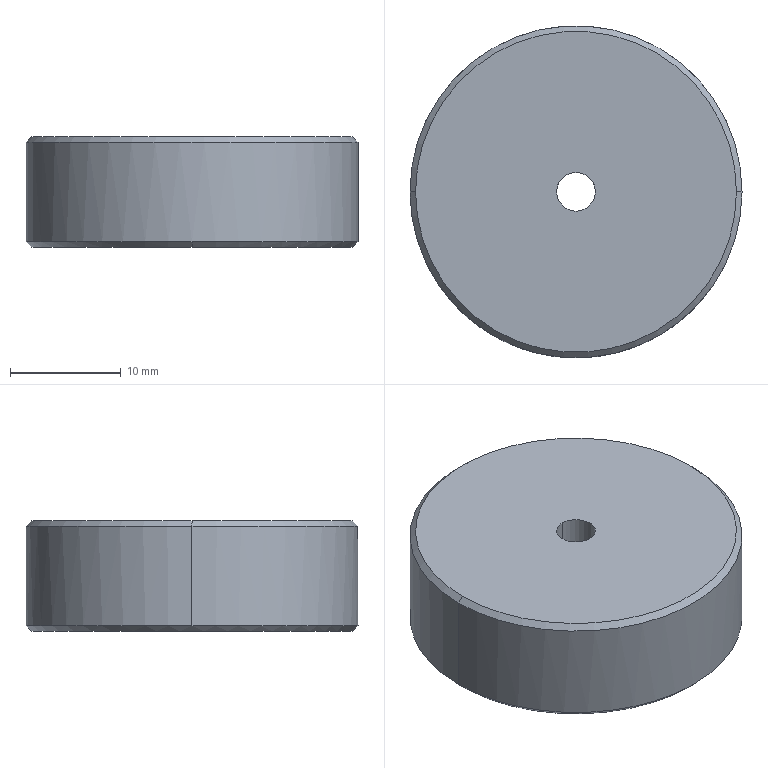Part | STEP file | 04-15 Heat-shrink tube press block | 1 solid | 15 faces | box 30 x 30 x 10 mm | volume 6743 mm3 | cone 6 | cylinder 6 | plane 3 | commonest cylinder face diameters 3.5 x2 8 x2 30 x2
STEP:
#1=CARTESIAN_POINT('',(0.,0.,0.));
#2=DIRECTION('',(0.,0.,1.));
#3=DIRECTION('',(1.,0.,0.));
#4=AXIS2_PLACEMENT_3D('',#1,#2,#3);
#5=CARTESIAN_POINT('',(14.5,0.,0.));
#6=VERTEX_POINT('',#5);
#7=CARTESIAN_POINT('',(-14.5,0.,0.));
#8=VERTEX_POINT('',#7);
#9=CARTESIAN_POINT('',(0.,0.,0.));
#10=DIRECTION('',(0.,0.,1.));
#11=DIRECTION('',(-1.,0.,0.));
#12=AXIS2_PLACEMENT_3D('',#9,#10,#11);
#13=CIRCLE('',#12,14.5);
#14=CARTESIAN_POINT('',(0.,0.,0.));
#15=DIRECTION('',(0.,0.,-1.));
#16=DIRECTION('',(-1.,0.,0.));
#17=AXIS2_PLACEMENT_3D('',#14,#15,#16);
#18=CONICAL_SURFACE('',#17,14.5,0.7854);
#19=CARTESIAN_POINT('',(6.283,0.));
#20=DIRECTION('',(-1.,0.));
#21=VECTOR('',#20,1.);
#22=LINE('',#19,#21);
#23=(GEOMETRIC_REPRESENTATION_CONTEXT(2)PARAMETRIC_REPRESENTATION_CONTEXT()REPRESENTATION_CONTEXT('',''));
#24=DEFINITIONAL_REPRESENTATION('',(#22),#23);
#25=PCURVE('',#18,#24);
#26=CARTESIAN_POINT('',(14.674,-14.674,0.));
#27=DIRECTION('',(0.,0.,-1.));
#28=DIRECTION('',(-1.,0.,0.));
#29=AXIS2_PLACEMENT_3D('',#26,#27,#28);
#30=PLANE('',#29);
#31=CARTESIAN_POINT('',(29.174,14.674));
#32=CARTESIAN_POINT('',(29.174,-10.441));
#33=CARTESIAN_POINT('',(7.424,2.117));
#34=CARTESIAN_POINT('',(-14.326,14.674));
#35=CARTESIAN_POINT('',(7.424,27.231));
#36=CARTESIAN_POINT('',(29.174,39.789));
#37=CARTESIAN_POINT('',(29.174,14.674));
#38=(BOUNDED_CURVE()B_SPLINE_CURVE(2,(#31,#32,#33,#34,#35,#36,#37),.UNSPECIFIED.,.T.,.F.)B_SPLINE_CURVE_WITH_KNOTS((1,2,2,2,2,1),(-2.094,0.,2.094,4.189,6.283,8.378),.UNSPECIFIED.)CURVE()GEOMETRIC_REPRESENTATION_ITEM()RATIONAL_B_SPLINE_CURVE((1.,0.5,1.,0.5,1.,0.5,1.))REPRESENTATION_ITEM(''));
#39=(GEOMETRIC_REPRESENTATION_CONTEXT(2)PARAMETRIC_REPRESENTATION_CONTEXT()REPRESENTATION_CONTEXT('',''));
#40=DEFINITIONAL_REPRESENTATION('',(#38),#39);
#41=PCURVE('',#30,#40);
#42=SURFACE_CURVE('',#13,(#25,#41),.PCURVE_S1.);
#43=EDGE_CURVE('',#6,#8,#42,.T.);
#44=ORIENTED_EDGE('',*,*,#43,.F.);
#45=CARTESIAN_POINT('',(15.,0.,-0.5));
#46=VERTEX_POINT('',#45);
#47=CARTESIAN_POINT('',(14.5,0.,0.));
#48=DIRECTION('',(0.7071,0.,-0.7071));
#49=VECTOR('',#48,1.);
#50=LINE('',#47,#49);
#51=CARTESIAN_POINT('',(3.142,0.));
#52=DIRECTION('',(0.,1.));
#53=VECTOR('',#52,1.);
#54=LINE('',#51,#53);
#55=(GEOMETRIC_REPRESENTATION_CONTEXT(2)PARAMETRIC_REPRESENTATION_CONTEXT()REPRESENTATION_CONTEXT('',''));
#56=DEFINITIONAL_REPRESENTATION('',(#54),#55);
#57=PCURVE('',#18,#56);
#58=CARTESIAN_POINT('',(0.,0.,0.));
#59=DIRECTION('',(0.,0.,-1.));
#60=DIRECTION('',(-1.,0.,0.));
#61=AXIS2_PLACEMENT_3D('',#58,#59,#60);
#62=CONICAL_SURFACE('',#61,14.5,0.7854);
#63=CARTESIAN_POINT('',(3.142,0.));
#64=DIRECTION('',(0.,1.));
#65=VECTOR('',#64,1.);
#66=LINE('',#63,#65);
#67=(GEOMETRIC_REPRESENTATION_CONTEXT(2)PARAMETRIC_REPRESENTATION_CONTEXT()REPRESENTATION_CONTEXT('',''));
#68=DEFINITIONAL_REPRESENTATION('',(#66),#67);
#69=PCURVE('',#62,#68);
#70=SURFACE_CURVE('',#50,(#57,#69),.PCURVE_S1.);
#71=EDGE_CURVE('',#6,#46,#70,.T.);
#72=ORIENTED_EDGE('',*,*,#71,.T.);
#73=CARTESIAN_POINT('',(-15.,0.,-0.5));
#74=VERTEX_POINT('',#73);
#75=CARTESIAN_POINT('',(0.,0.,-0.5));
#76=DIRECTION('',(0.,0.,-1.));
#77=DIRECTION('',(-1.,0.,0.));
#78=AXIS2_PLACEMENT_3D('',#75,#76,#77);
#79=CIRCLE('',#78,15.);
#80=CARTESIAN_POINT('',(0.,0.5));
#81=DIRECTION('',(1.,0.));
#82=VECTOR('',#81,1.);
#83=LINE('',#80,#82);
#84=(GEOMETRIC_REPRESENTATION_CONTEXT(2)PARAMETRIC_REPRESENTATION_CONTEXT()REPRESENTATION_CONTEXT('',''));
#85=DEFINITIONAL_REPRESENTATION('',(#83),#84);
#86=PCURVE('',#18,#85);
#87=CARTESIAN_POINT('',(0.,0.,-9.5));
#88=DIRECTION('',(0.,0.,1.));
#89=DIRECTION('',(1.,0.,0.));
#90=AXIS2_PLACEMENT_3D('',#87,#88,#89);
#91=CYLINDRICAL_SURFACE('',#90,15.);
#92=CARTESIAN_POINT('',(3.142,9.));
#93=DIRECTION('',(-1.,0.));
#94=VECTOR('',#93,1.);
#95=LINE('',#92,#94);
#96=(GEOMETRIC_REPRESENTATION_CONTEXT(2)PARAMETRIC_REPRESENTATION_CONTEXT()REPRESENTATION_CONTEXT('',''));
#97=DEFINITIONAL_REPRESENTATION('',(#95),#96);
#98=PCURVE('',#91,#97);
#99=SURFACE_CURVE('',#79,(#86,#98),.PCURVE_S1.);
#100=EDGE_CURVE('',#74,#46,#99,.T.);
#101=ORIENTED_EDGE('',*,*,#100,.F.);
#102=CARTESIAN_POINT('',(-14.5,0.,0.));
#103=DIRECTION('',(-0.7071,0.,-0.7071));
#104=VECTOR('',#103,1.);
#105=LINE('',#102,#104);
#106=CARTESIAN_POINT('',(0.,0.));
#107=DIRECTION('',(0.,1.));
#108=VECTOR('',#107,1.);
#109=LINE('',#106,#108);
#110=(GEOMETRIC_REPRESENTATION_CONTEXT(2)PARAMETRIC_REPRESENTATION_CONTEXT()REPRESENTATION_CONTEXT('',''));
#111=DEFINITIONAL_REPRESENTATION('',(#109),#110);
#112=PCURVE('',#18,#111);
#113=CARTESIAN_POINT('',(6.283,0.));
#114=DIRECTION('',(0.,1.));
#115=VECTOR('',#114,1.);
#116=LINE('',#113,#115);
#117=(GEOMETRIC_REPRESENTATION_CONTEXT(2)PARAMETRIC_REPRESENTATION_CONTEXT()REPRESENTATION_CONTEXT('',''));
#118=DEFINITIONAL_REPRESENTATION('',(#116),#117);
#119=PCURVE('',#62,#118);
#120=SURFACE_CURVE('',#105,(#112,#119),.PCURVE_S1.);
#121=EDGE_CURVE('',#8,#74,#120,.T.);
#122=ORIENTED_EDGE('',*,*,#121,.F.);
#123=EDGE_LOOP('',(#44,#72,#101,#122));
#124=FACE_BOUND('',#123,.T.);
#125=ADVANCED_FACE('',(#124),#18,.T.);
#126=CARTESIAN_POINT('',(-15.,0.,-9.5));
#127=VERTEX_POINT('',#126);
#128=CARTESIAN_POINT('',(0.,15.,-9.5));
#129=VERTEX_POINT('',#128);
#130=CARTESIAN_POINT('',(0.,0.,-9.5));
#131=DIRECTION('',(0.,0.,-1.));
#132=DIRECTION('',(1.,0.,0.));
#133=AXIS2_PLACEMENT_3D('',#130,#131,#132);
#134=CIRCLE('',#133,15.);
#135=CARTESIAN_POINT('',(6.283,0.));
#136=DIRECTION('',(-1.,0.));
#137=VECTOR('',#136,1.);
#138=LINE('',#135,#137);
#139=(GEOMETRIC_REPRESENTATION_CONTEXT(2)PARAMETRIC_REPRESENTATION_CONTEXT()REPRESENTATION_CONTEXT('',''));
#140=DEFINITIONAL_REPRESENTATION('',(#138),#139);
#141=PCURVE('',#91,#140);
#142=CARTESIAN_POINT('',(0.,0.,-10.));
#143=DIRECTION('',(0.,0.,1.));
#144=DIRECTION('',(0.,-1.,0.));
#145=AXIS2_PLACEMENT_3D('',#142,#143,#144);
#146=CONICAL_SURFACE('',#145,14.5,0.7854);
#147=CARTESIAN_POINT('',(7.854,0.5));
#148=DIRECTION('',(-1.,0.));
#149=VECTOR('',#148,1.);
#150=LINE('',#147,#149);
#151=(GEOMETRIC_REPRESENTATION_CONTEXT(2)PARAMETRIC_REPRESENTATION_CONTEXT()REPRESENTATION_CONTEXT('',''));
#152=DEFINITIONAL_REPRESENTATION('',(#150),#151);
#153=PCURVE('',#146,#152);
#154=SURFACE_CURVE('',#134,(#141,#153),.PCURVE_S1.);
#155=EDGE_CURVE('',#127,#129,#154,.T.);
#156=ORIENTED_EDGE('',*,*,#155,.F.);
#157=CARTESIAN_POINT('',(-15.,0.,-9.5));
#158=DIRECTION('',(0.,0.,1.));
#159=VECTOR('',#158,1.);
#160=LINE('',#157,#159);
#161=CARTESIAN_POINT('',(3.142,0.));
#162=DIRECTION('',(0.,1.));
#163=VECTOR('',#162,1.);
#164=LINE('',#161,#163);
#165=(GEOMETRIC_REPRESENTATION_CONTEXT(2)PARAMETRIC_REPRESENTATION_CONTEXT()REPRESENTATION_CONTEXT('',''));
#166=DEFINITIONAL_REPRESENTATION('',(#164),#165);
#167=PCURVE('',#91,#166);
#168=CARTESIAN_POINT('',(0.,0.,-9.5));
#169=DIRECTION('',(0.,0.,1.));
#170=DIRECTION('',(1.,0.,0.));
#171=AXIS2_PLACEMENT_3D('',#168,#169,#170);
#172=CYLINDRICAL_SURFACE('',#171,15.);
#173=CARTESIAN_POINT('',(3.142,0.));
#174=DIRECTION('',(0.,1.));
#175=VECTOR('',#174,1.);
#176=LINE('',#173,#175);
#177=(GEOMETRIC_REPRESENTATION_CONTEXT(2)PARAMETRIC_REPRESENTATION_CONTEXT()REPRESENTATION_CONTEXT('',''));
#178=DEFINITIONAL_REPRESENTATION('',(#176),#177);
#179=PCURVE('',#172,#178);
#180=SURFACE_CURVE('',#160,(#167,#179),.PCURVE_S1.);
#181=EDGE_CURVE('',#127,#74,#180,.T.);
#182=ORIENTED_EDGE('',*,*,#181,.T.);
#183=ORIENTED_EDGE('',*,*,#100,.T.);
#184=CARTESIAN_POINT('',(15.,0.,-9.5));
#185=VERTEX_POINT('',#184);
#186=CARTESIAN_POINT('',(15.,0.,-9.5));
#187=DIRECTION('',(0.,0.,1.));
#188=VECTOR('',#187,1.);
#189=LINE('',#186,#188);
#190=CARTESIAN_POINT('',(0.,0.));
#191=DIRECTION('',(0.,1.));
#192=VECTOR('',#191,1.);
#193=LINE('',#190,#192);
#194=(GEOMETRIC_REPRESENTATION_CONTEXT(2)PARAMETRIC_REPRESENTATION_CONTEXT()REPRESENTATION_CONTEXT('',''));
#195=DEFINITIONAL_REPRESENTATION('',(#193),#194);
#196=PCURVE('',#91,#195);
#197=CARTESIAN_POINT('',(6.283,0.));
#198=DIRECTION('',(0.,1.));
#199=VECTOR('',#198,1.);
#200=LINE('',#197,#199);
#201=(GEOMETRIC_REPRESENTATION_CONTEXT(2)PARAMETRIC_REPRESENTATION_CONTEXT()REPRESENTATION_CONTEXT('',''));
#202=DEFINITIONAL_REPRESENTATION('',(#200),#201);
#203=PCURVE('',#172,#202);
#204=SURFACE_CURVE('',#189,(#196,#203),.PCURVE_S1.);
#205=EDGE_CURVE('',#185,#46,#204,.T.);
#206=ORIENTED_EDGE('',*,*,#205,.F.);
#207=CARTESIAN_POINT('',(0.,0.,-9.5));
#208=DIRECTION('',(0.,0.,-1.));
#209=DIRECTION('',(1.,0.,0.));
#210=AXIS2_PLACEMENT_3D('',#207,#208,#209);
#211=CIRCLE('',#210,15.);
#212=CARTESIAN_POINT('',(6.283,0.));
#213=DIRECTION('',(-1.,0.));
#214=VECTOR('',#213,1.);
#215=LINE('',#212,#214);
#216=(GEOMETRIC_REPRESENTATION_CONTEXT(2)PARAMETRIC_REPRESENTATION_CONTEXT()REPRESENTATION_CONTEXT('',''));
#217=DEFINITIONAL_REPRESENTATION('',(#215),#216);
#218=PCURVE('',#91,#217);
#219=CARTESIAN_POINT('',(0.,0.,-10.));
#220=DIRECTION('',(0.,0.,1.));
#221=DIRECTION('',(0.,-1.,0.));
#222=AXIS2_PLACEMENT_3D('',#219,#220,#221);
#223=CONICAL_SURFACE('',#222,14.5,0.7854);
#224=CARTESIAN_POINT('',(7.854,0.5));
#225=DIRECTION('',(-1.,0.));
#226=VECTOR('',#225,1.);
#227=LINE('',#224,#226);
#228=(GEOMETRIC_REPRESENTATION_CONTEXT(2)PARAMETRIC_REPRESENTATION_CONTEXT()REPRESENTATION_CONTEXT('',''));
#229=DEFINITIONAL_REPRESENTATION('',(#227),#228);
#230=PCURVE('',#223,#229);
#231=SURFACE_CURVE('',#211,(#218,#230),.PCURVE_S1.);
#232=EDGE_CURVE('',#129,#185,#231,.T.);
#233=ORIENTED_EDGE('',*,*,#232,.F.);
#234=EDGE_LOOP('',(#156,#182,#183,#206,#233));
#235=FACE_BOUND('',#234,.T.);
#236=ADVANCED_FACE('',(#235),#91,.T.);
#237=CARTESIAN_POINT('',(0.,-1.75,-5.));
#238=VERTEX_POINT('',#237);
#239=CARTESIAN_POINT('',(0.,-1.75,0.));
#240=VERTEX_POINT('',#239);
#241=CARTESIAN_POINT('',(0.,-1.75,-5.));
#242=DIRECTION('',(0.,0.,1.));
#243=VECTOR('',#242,1.);
#244=LINE('',#241,#243);
#245=CARTESIAN_POINT('',(0.,0.,-5.));
#246=DIRECTION('',(0.,0.,1.));
#247=DIRECTION('',(0.,-1.,0.));
#248=AXIS2_PLACEMENT_3D('',#245,#246,#247);
#249=CYLINDRICAL_SURFACE('',#248,1.75);
#250=CARTESIAN_POINT('',(6.283,0.));
#251=DIRECTION('',(0.,1.));
#252=VECTOR('',#251,1.);
#253=LINE('',#250,#252);
#254=(GEOMETRIC_REPRESENTATION_CONTEXT(2)PARAMETRIC_REPRESENTATION_CONTEXT()REPRESENTATION_CONTEXT('',''));
#255=DEFINITIONAL_REPRESENTATION('',(#253),#254);
#256=PCURVE('',#249,#255);
#257=CARTESIAN_POINT('',(0.,0.,-5.));
#258=DIRECTION('',(0.,0.,1.));
#259=DIRECTION('',(0.,-1.,0.));
#260=AXIS2_PLACEMENT_3D('',#257,#258,#259);
#261=CYLINDRICAL_SURFACE('',#260,1.75);
#262=CARTESIAN_POINT('',(0.,0.));
#263=DIRECTION('',(0.,1.));
#264=VECTOR('',#263,1.);
#265=LINE('',#262,#264);
#266=(GEOMETRIC_REPRESENTATION_CONTEXT(2)PARAMETRIC_REPRESENTATION_CONTEXT()REPRESENTATION_CONTEXT('',''));
#267=DEFINITIONAL_REPRESENTATION('',(#265),#266);
#268=PCURVE('',#261,#267);
#269=SURFACE_CURVE('',#244,(#256,#268),.PCURVE_S1.);
#270=EDGE_CURVE('',#238,#240,#269,.T.);
#271=ORIENTED_EDGE('',*,*,#270,.T.);
#272=CARTESIAN_POINT('',(0.,1.75,0.));
#273=VERTEX_POINT('',#272);
#274=CARTESIAN_POINT('',(0.,0.,0.));
#275=DIRECTION('',(0.,0.,1.));
#276=DIRECTION('',(0.,-1.,0.));
#277=AXIS2_PLACEMENT_3D('',#274,#275,#276);
#278=CIRCLE('',#277,1.75);
#279=CARTESIAN_POINT('',(0.,5.));
#280=DIRECTION('',(1.,0.));
#281=VECTOR('',#280,1.);
#282=LINE('',#279,#281);
#283=(GEOMETRIC_REPRESENTATION_CONTEXT(2)PARAMETRIC_REPRESENTATION_CONTEXT()REPRESENTATION_CONTEXT('',''));
#284=DEFINITIONAL_REPRESENTATION('',(#282),#283);
#285=PCURVE('',#249,#284);
#286=CARTESIAN_POINT('',(14.674,12.924));
#287=CARTESIAN_POINT('',(11.643,12.924));
#288=CARTESIAN_POINT('',(13.158,15.549));
#289=CARTESIAN_POINT('',(14.674,18.174));
#290=CARTESIAN_POINT('',(16.19,15.549));
#291=CARTESIAN_POINT('',(17.705,12.924));
#292=CARTESIAN_POINT('',(14.674,12.924));
#293=(BOUNDED_CURVE()B_SPLINE_CURVE(2,(#286,#287,#288,#289,#290,#291,#292),.UNSPECIFIED.,.T.,.F.)B_SPLINE_CURVE_WITH_KNOTS((1,2,2,2,2,1),(-2.094,0.,2.094,4.189,6.283,8.378),.UNSPECIFIED.)CURVE()GEOMETRIC_REPRESENTATION_ITEM()RATIONAL_B_SPLINE_CURVE((1.,0.5,1.,0.5,1.,0.5,1.))REPRESENTATION_ITEM(''));
#294=(GEOMETRIC_REPRESENTATION_CONTEXT(2)PARAMETRIC_REPRESENTATION_CONTEXT()REPRESENTATION_CONTEXT('',''));
#295=DEFINITIONAL_REPRESENTATION('',(#293),#294);
#296=PCURVE('',#30,#295);
#297=SURFACE_CURVE('',#278,(#285,#296),.PCURVE_S1.);
#298=EDGE_CURVE('',#273,#240,#297,.T.);
#299=ORIENTED_EDGE('',*,*,#298,.F.);
#300=CARTESIAN_POINT('',(0.,1.75,-5.));
#301=VERTEX_POINT('',#300);
#302=CARTESIAN_POINT('',(0.,1.75,-5.));
#303=DIRECTION('',(0.,0.,1.));
#304=VECTOR('',#303,1.);
#305=LINE('',#302,#304);
#306=CARTESIAN_POINT('',(3.142,0.));
#307=DIRECTION('',(0.,1.));
#308=VECTOR('',#307,1.);
#309=LINE('',#306,#308);
#310=(GEOMETRIC_REPRESENTATION_CONTEXT(2)PARAMETRIC_REPRESENTATION_CONTEXT()REPRESENTATION_CONTEXT('',''));
#311=DEFINITIONAL_REPRESENTATION('',(#309),#310);
#312=PCURVE('',#249,#311);
#313=CARTESIAN_POINT('',(3.142,0.));
#314=DIRECTION('',(0.,1.));
#315=VECTOR('',#314,1.);
#316=LINE('',#313,#315);
#317=(GEOMETRIC_REPRESENTATION_CONTEXT(2)PARAMETRIC_REPRESENTATION_CONTEXT()REPRESENTATION_CONTEXT('',''));
#318=DEFINITIONAL_REPRESENTATION('',(#316),#317);
#319=PCURVE('',#261,#318);
#320=SURFACE_CURVE('',#305,(#312,#319),.PCURVE_S1.);
#321=EDGE_CURVE('',#301,#273,#320,.T.);
#322=ORIENTED_EDGE('',*,*,#321,.F.);
#323=CARTESIAN_POINT('',(0.,0.,-5.));
#324=DIRECTION('',(0.,0.,-1.));
#325=DIRECTION('',(0.,-1.,0.));
#326=AXIS2_PLACEMENT_3D('',#323,#324,#325);
#327=CIRCLE('',#326,1.75);
#328=CARTESIAN_POINT('',(6.283,0.));
#329=DIRECTION('',(-1.,0.));
#330=VECTOR('',#329,1.);
#331=LINE('',#328,#330);
#332=(GEOMETRIC_REPRESENTATION_CONTEXT(2)PARAMETRIC_REPRESENTATION_CONTEXT()REPRESENTATION_CONTEXT('',''));
#333=DEFINITIONAL_REPRESENTATION('',(#331),#332);
#334=PCURVE('',#249,#333);
#335=CARTESIAN_POINT('',(-4.048,-4.048,-5.));
#336=DIRECTION('',(0.,0.,1.));
#337=DIRECTION('',(1.,0.,0.));
#338=AXIS2_PLACEMENT_3D('',#335,#336,#337);
#339=PLANE('',#338);
#340=CARTESIAN_POINT('',(4.048,2.298));
#341=CARTESIAN_POINT('',(1.017,2.298));
#342=CARTESIAN_POINT('',(2.532,4.923));
#343=CARTESIAN_POINT('',(4.048,7.548));
#344=CARTESIAN_POINT('',(5.564,4.923));
#345=CARTESIAN_POINT('',(7.079,2.298));
#346=CARTESIAN_POINT('',(4.048,2.298));
#347=(BOUNDED_CURVE()B_SPLINE_CURVE(2,(#340,#341,#342,#343,#344,#345,#346),.UNSPECIFIED.,.T.,.F.)B_SPLINE_CURVE_WITH_KNOTS((1,2,2,2,2,1),(-2.094,0.,2.094,4.189,6.283,8.378),.UNSPECIFIED.)CURVE()GEOMETRIC_REPRESENTATION_ITEM()RATIONAL_B_SPLINE_CURVE((1.,0.5,1.,0.5,1.,0.5,1.))REPRESENTATION_ITEM(''));
#348=(GEOMETRIC_REPRESENTATION_CONTEXT(2)PARAMETRIC_REPRESENTATION_CONTEXT()REPRESENTATION_CONTEXT('',''));
#349=DEFINITIONAL_REPRESENTATION('',(#347),#348);
#350=PCURVE('',#339,#349);
#351=SURFACE_CURVE('',#327,(#334,#350),.PCURVE_S1.);
#352=EDGE_CURVE('',#238,#301,#351,.T.);
#353=ORIENTED_EDGE('',*,*,#352,.F.);
#354=EDGE_LOOP('',(#271,#299,#322,#353));
#355=FACE_BOUND('',#354,.F.);
#356=ADVANCED_FACE('',(#355),#249,.F.);
#357=CARTESIAN_POINT('',(0.,14.5,-10.));
#358=VERTEX_POINT('',#357);
#359=CARTESIAN_POINT('',(0.,-14.5,-10.));
#360=VERTEX_POINT('',#359);
#361=CARTESIAN_POINT('',(0.,0.,-10.));
#362=DIRECTION('',(0.,0.,-1.));
#363=DIRECTION('',(0.,-1.,0.));
#364=AXIS2_PLACEMENT_3D('',#361,#362,#363);
#365=CIRCLE('',#364,14.5);
#366=CARTESIAN_POINT('',(6.283,0.));
#367=DIRECTION('',(-1.,0.));
#368=VECTOR('',#367,1.);
#369=LINE('',#366,#368);
#370=(GEOMETRIC_REPRESENTATION_CONTEXT(2)PARAMETRIC_REPRESENTATION_CONTEXT()REPRESENTATION_CONTEXT('',''));
#371=DEFINITIONAL_REPRESENTATION('',(#369),#370);
#372=PCURVE('',#223,#371);
#373=CARTESIAN_POINT('',(-14.674,-14.674,-10.));
#374=DIRECTION('',(0.,0.,1.));
#375=DIRECTION('',(1.,0.,0.));
#376=AXIS2_PLACEMENT_3D('',#373,#374,#375);
#377=PLANE('',#376);
#378=CARTESIAN_POINT('',(14.674,0.174));
#379=CARTESIAN_POINT('',(-10.441,0.174));
#380=CARTESIAN_POINT('',(2.117,21.924));
#381=CARTESIAN_POINT('',(14.674,43.674));
#382=CARTESIAN_POINT('',(27.231,21.924));
#383=CARTESIAN_POINT('',(39.789,0.174));
#384=CARTESIAN_POINT('',(14.674,0.174));
#385=(BOUNDED_CURVE()B_SPLINE_CURVE(2,(#378,#379,#380,#381,#382,#383,#384),.UNSPECIFIED.,.T.,.F.)B_SPLINE_CURVE_WITH_KNOTS((1,2,2,2,2,1),(-2.094,0.,2.094,4.189,6.283,8.378),.UNSPECIFIED.)CURVE()GEOMETRIC_REPRESENTATION_ITEM()RATIONAL_B_SPLINE_CURVE((1.,0.5,1.,0.5,1.,0.5,1.))REPRESENTATION_ITEM(''));
#386=(GEOMETRIC_REPRESENTATION_CONTEXT(2)PARAMETRIC_REPRESENTATION_CONTEXT()REPRESENTATION_CONTEXT('',''));
#387=DEFINITIONAL_REPRESENTATION('',(#385),#386);
#388=PCURVE('',#377,#387);
#389=SURFACE_CURVE('',#365,(#372,#388),.PCURVE_S1.);
#390=EDGE_CURVE('',#358,#360,#389,.T.);
#391=ORIENTED_EDGE('',*,*,#390,.F.);
#392=CARTESIAN_POINT('',(0.,14.5,-10.));
#393=DIRECTION('',(0.,0.7071,0.7071));
#394=VECTOR('',#393,1.);
#395=LINE('',#392,#394);
#396=CARTESIAN_POINT('',(3.142,0.));
#397=DIRECTION('',(0.,1.));
#398=VECTOR('',#397,1.);
#399=LINE('',#396,#398);
#400=(GEOMETRIC_REPRESENTATION_CONTEXT(2)PARAMETRIC_REPRESENTATION_CONTEXT()REPRESENTATION_CONTEXT('',''));
#401=DEFINITIONAL_REPRESENTATION('',(#399),#400);
#402=PCURVE('',#223,#401);
#403=CARTESIAN_POINT('',(3.142,0.));
#404=DIRECTION('',(0.,1.));
#405=VECTOR('',#404,1.);
#406=LINE('',#403,#405);
#407=(GEOMETRIC_REPRESENTATION_CONTEXT(2)PARAMETRIC_REPRESENTATION_CONTEXT()REPRESENTATION_CONTEXT('',''));
#408=DEFINITIONAL_REPRESENTATION('',(#406),#407);
#409=PCURVE('',#146,#408);
#410=SURFACE_CURVE('',#395,(#402,#409),.PCURVE_S1.);
#411=EDGE_CURVE('',#358,#129,#410,.T.);
#412=ORIENTED_EDGE('',*,*,#411,.T.);
#413=ORIENTED_EDGE('',*,*,#232,.T.);
#414=CARTESIAN_POINT('',(0.,-15.,-9.5));
#415=VERTEX_POINT('',#414);
#416=CARTESIAN_POINT('',(0.,0.,-9.5));
#417=DIRECTION('',(0.,0.,-1.));
#418=DIRECTION('',(1.,0.,0.));
#419=AXIS2_PLACEMENT_3D('',#416,#417,#418);
#420=CIRCLE('',#419,15.);
#421=CARTESIAN_POINT('',(1.571,0.5));
#422=DIRECTION('',(-1.,0.));
#423=VECTOR('',#422,1.);
#424=LINE('',#421,#423);
#425=(GEOMETRIC_REPRESENTATION_CONTEXT(2)PARAMETRIC_REPRESENTATION_CONTEXT()REPRESENTATION_CONTEXT('',''));
#426=DEFINITIONAL_REPRESENTATION('',(#424),#425);
#427=PCURVE('',#223,#426);
#428=CARTESIAN_POINT('',(6.283,0.));
#429=DIRECTION('',(-1.,0.));
#430=VECTOR('',#429,1.);
#431=LINE('',#428,#430);
#432=(GEOMETRIC_REPRESENTATION_CONTEXT(2)PARAMETRIC_REPRESENTATION_CONTEXT()REPRESENTATION_CONTEXT('',''));
#433=DEFINITIONAL_REPRESENTATION('',(#431),#432);
#434=PCURVE('',#172,#433);
#435=SURFACE_CURVE('',#420,(#427,#434),.PCURVE_S1.);
#436=EDGE_CURVE('',#185,#415,#435,.T.);
#437=ORIENTED_EDGE('',*,*,#436,.T.);
#438=CARTESIAN_POINT('',(0.,-14.5,-10.));
#439=DIRECTION('',(0.,-0.7071,0.7071));
#440=VECTOR('',#439,1.);
#441=LINE('',#438,#440);
#442=CARTESIAN_POINT('',(0.,0.));
#443=DIRECTION('',(0.,1.));
#444=VECTOR('',#443,1.);
#445=LINE('',#442,#444);
#446=(GEOMETRIC_REPRESENTATION_CONTEXT(2)PARAMETRIC_REPRESENTATION_CONTEXT()REPRESENTATION_CONTEXT('',''));
#447=DEFINITIONAL_REPRESENTATION('',(#445),#446);
#448=PCURVE('',#223,#447);
#449=CARTESIAN_POINT('',(6.283,0.));
#450=DIRECTION('',(0.,1.));
#451=VECTOR('',#450,1.);
#452=LINE('',#449,#451);
#453=(GEOMETRIC_REPRESENTATION_CONTEXT(2)PARAMETRIC_REPRESENTATION_CONTEXT()REPRESENTATION_CONTEXT('',''));
#454=DEFINITIONAL_REPRESENTATION('',(#452),#453);
#455=PCURVE('',#146,#454);
#456=SURFACE_CURVE('',#441,(#448,#455),.PCURVE_S1.);
#457=EDGE_CURVE('',#360,#415,#456,.T.);
#458=ORIENTED_EDGE('',*,*,#457,.F.);
#459=EDGE_LOOP('',(#391,#412,#413,#437,#458));
#460=FACE_BOUND('',#459,.T.);
#461=ADVANCED_FACE('',(#460),#223,.T.);
#462=CARTESIAN_POINT('',(4.,0.,-9.5));
#463=VERTEX_POINT('',#462);
#464=CARTESIAN_POINT('',(4.,0.,-5.));
#465=VERTEX_POINT('',#464);
#466=CARTESIAN_POINT('',(4.,0.,-9.5));
#467=DIRECTION('',(0.,0.,1.));
#468=VECTOR('',#467,1.);
#469=LINE('',#466,#468);
#470=CARTESIAN_POINT('',(0.,0.,-9.5));
#471=DIRECTION('',(0.,0.,1.));
#472=DIRECTION('',(1.,0.,0.));
#473=AXIS2_PLACEMENT_3D('',#470,#471,#472);
#474=CYLINDRICAL_SURFACE('',#473,4.);
#475=CARTESIAN_POINT('',(6.283,0.));
#476=DIRECTION('',(0.,1.));
#477=VECTOR('',#476,1.);
#478=LINE('',#475,#477);
#479=(GEOMETRIC_REPRESENTATION_CONTEXT(2)PARAMETRIC_REPRESENTATION_CONTEXT()REPRESENTATION_CONTEXT('',''));
#480=DEFINITIONAL_REPRESENTATION('',(#478),#479);
#481=PCURVE('',#474,#480);
#482=CARTESIAN_POINT('',(0.,0.,-9.5));
#483=DIRECTION('',(0.,0.,1.));
#484=DIRECTION('',(1.,0.,0.));
#485=AXIS2_PLACEMENT_3D('',#482,#483,#484);
#486=CYLINDRICAL_SURFACE('',#485,4.);
#487=CARTESIAN_POINT('',(0.,0.));
#488=DIRECTION('',(0.,1.));
#489=VECTOR('',#488,1.);
#490=LINE('',#487,#489);
#491=(GEOMETRIC_REPRESENTATION_CONTEXT(2)PARAMETRIC_REPRESENTATION_CONTEXT()REPRESENTATION_CONTEXT('',''));
#492=DEFINITIONAL_REPRESENTATION('',(#490),#491);
#493=PCURVE('',#486,#492);
#494=SURFACE_CURVE('',#469,(#481,#493),.PCURVE_S1.);
#495=EDGE_CURVE('',#463,#465,#494,.T.);
#496=ORIENTED_EDGE('',*,*,#495,.T.);
#497=CARTESIAN_POINT('',(-4.,0.,-5.));
#498=VERTEX_POINT('',#497);
#499=CARTESIAN_POINT('',(0.,0.,-5.));
#500=DIRECTION('',(0.,0.,1.));
#501=DIRECTION('',(1.,0.,0.));
#502=AXIS2_PLACEMENT_3D('',#499,#500,#501);
#503=CIRCLE('',#502,4.);
#504=CARTESIAN_POINT('',(0.,4.5));
#505=DIRECTION('',(1.,0.));
#506=VECTOR('',#505,1.);
#507=LINE('',#504,#506);
#508=(GEOMETRIC_REPRESENTATION_CONTEXT(2)PARAMETRIC_REPRESENTATION_CONTEXT()REPRESENTATION_CONTEXT('',''));
#509=DEFINITIONAL_REPRESENTATION('',(#507),#508);
#510=PCURVE('',#474,#509);
#511=CARTESIAN_POINT('',(4.048,4.048));
#512=DIRECTION('',(1.,0.));
#513=AXIS2_PLACEMENT_2D('',#511,#512);
#514=CIRCLE('',#513,4.);
#515=(GEOMETRIC_REPRESENTATION_CONTEXT(2)PARAMETRIC_REPRESENTATION_CONTEXT()REPRESENTATION_CONTEXT('',''));
#516=DEFINITIONAL_REPRESENTATION('',(#514),#515);
#517=PCURVE('',#339,#516);
#518=SURFACE_CURVE('',#503,(#510,#517),.PCURVE_S1.);
#519=EDGE_CURVE('',#498,#465,#518,.T.);
#520=ORIENTED_EDGE('',*,*,#519,.F.);
#521=CARTESIAN_POINT('',(-4.,0.,-9.5));
#522=VERTEX_POINT('',#521);
#523=CARTESIAN_POINT('',(-4.,0.,-9.5));
#524=DIRECTION('',(0.,0.,1.));
#525=VECTOR('',#524,1.);
#526=LINE('',#523,#525);
#527=CARTESIAN_POINT('',(3.142,0.));
#528=DIRECTION('',(0.,1.));
#529=VECTOR('',#528,1.);
#530=LINE('',#527,#529);
#531=(GEOMETRIC_REPRESENTATION_CONTEXT(2)PARAMETRIC_REPRESENTATION_CONTEXT()REPRESENTATION_CONTEXT('',''));
#532=DEFINITIONAL_REPRESENTATION('',(#530),#531);
#533=PCURVE('',#474,#532);
#534=CARTESIAN_POINT('',(3.142,0.));
#535=DIRECTION('',(0.,1.));
#536=VECTOR('',#535,1.);
#537=LINE('',#534,#536);
#538=(GEOMETRIC_REPRESENTATION_CONTEXT(2)PARAMETRIC_REPRESENTATION_CONTEXT()REPRESENTATION_CONTEXT('',''));
#539=DEFINITIONAL_REPRESENTATION('',(#537),#538);
#540=PCURVE('',#486,#539);
#541=SURFACE_CURVE('',#526,(#533,#540),.PCURVE_S1.);
#542=EDGE_CURVE('',#522,#498,#541,.T.);
#543=ORIENTED_EDGE('',*,*,#542,.F.);
#544=CARTESIAN_POINT('',(0.,0.,-9.5));
#545=DIRECTION('',(0.,0.,-1.));
#546=DIRECTION('',(1.,0.,0.));
#547=AXIS2_PLACEMENT_3D('',#544,#545,#546);
#548=CIRCLE('',#547,4.);
#549=CARTESIAN_POINT('',(6.283,0.));
#550=DIRECTION('',(-1.,0.));
#551=VECTOR('',#550,1.);
#552=LINE('',#549,#551);
#553=(GEOMETRIC_REPRESENTATION_CONTEXT(2)PARAMETRIC_REPRESENTATION_CONTEXT()REPRESENTATION_CONTEXT('',''));
#554=DEFINITIONAL_REPRESENTATION('',(#552),#553);
#555=PCURVE('',#474,#554);
#556=CARTESIAN_POINT('',(0.,0.,-9.5));
#557=DIRECTION('',(0.,0.,-1.));
#558=DIRECTION('',(-1.,0.,0.));
#559=AXIS2_PLACEMENT_3D('',#556,#557,#558);
#560=CONICAL_SURFACE('',#559,4.,0.7854);
#561=CARTESIAN_POINT('',(3.142,0.));
#562=DIRECTION('',(1.,0.));
#563=VECTOR('',#562,1.);
#564=LINE('',#561,#563);
#565=(GEOMETRIC_REPRESENTATION_CONTEXT(2)PARAMETRIC_REPRESENTATION_CONTEXT()REPRESENTATION_CONTEXT('',''));
#566=DEFINITIONAL_REPRESENTATION('',(#564),#565);
#567=PCURVE('',#560,#566);
#568=SURFACE_CURVE('',#548,(#555,#567),.PCURVE_S1.);
#569=EDGE_CURVE('',#463,#522,#568,.T.);
#570=ORIENTED_EDGE('',*,*,#569,.F.);
#571=EDGE_LOOP('',(#496,#520,#543,#570));
#572=FACE_BOUND('',#571,.F.);
#573=ADVANCED_FACE('',(#572),#474,.F.);
#574=CARTESIAN_POINT('',(-4.5,0.,-10.));
#575=VERTEX_POINT('',#574);
#576=CARTESIAN_POINT('',(-4.,0.,-9.5));
#577=DIRECTION('',(-0.7071,0.,-0.7071));
#578=VECTOR('',#577,1.);
#579=LINE('',#576,#578);
#580=CARTESIAN_POINT('',(6.283,0.));
#581=DIRECTION('',(0.,1.));
#582=VECTOR('',#581,1.);
#583=LINE('',#580,#582);
#584=(GEOMETRIC_REPRESENTATION_CONTEXT(2)PARAMETRIC_REPRESENTATION_CONTEXT()REPRESENTATION_CONTEXT('',''));
#585=DEFINITIONAL_REPRESENTATION('',(#583),#584);
#586=PCURVE('',#560,#585);
#587=CARTESIAN_POINT('',(0.,0.,-9.5));
#588=DIRECTION('',(0.,0.,-1.));
#589=DIRECTION('',(-1.,0.,0.));
#590=AXIS2_PLACEMENT_3D('',#587,#588,#589);
#591=CONICAL_SURFACE('',#590,4.,0.7854);
#592=CARTESIAN_POINT('',(0.,0.));
#593=DIRECTION('',(0.,1.));
#594=VECTOR('',#593,1.);
#595=LINE('',#592,#594);
#596=(GEOMETRIC_REPRESENTATION_CONTEXT(2)PARAMETRIC_REPRESENTATION_CONTEXT()REPRESENTATION_CONTEXT('',''));
#597=DEFINITIONAL_REPRESENTATION('',(#595),#596);
#598=PCURVE('',#591,#597);
#599=SURFACE_CURVE('',#579,(#586,#598),.PCURVE_S1.);
#600=EDGE_CURVE('',#522,#575,#599,.T.);
#601=ORIENTED_EDGE('',*,*,#600,.T.);
#602=CARTESIAN_POINT('',(4.5,0.,-10.));
#603=VERTEX_POINT('',#602);
#604=CARTESIAN_POINT('',(0.,0.,-10.));
#605=DIRECTION('',(0.,0.,-1.));
#606=DIRECTION('',(-1.,0.,0.));
#607=AXIS2_PLACEMENT_3D('',#604,#605,#606);
#608=CIRCLE('',#607,4.5);
#609=CARTESIAN_POINT('',(0.,0.5));
#610=DIRECTION('',(1.,0.));
#611=VECTOR('',#610,1.);
#612=LINE('',#609,#611);
#613=(GEOMETRIC_REPRESENTATION_CONTEXT(2)PARAMETRIC_REPRESENTATION_CONTEXT()REPRESENTATION_CONTEXT('',''));
#614=DEFINITIONAL_REPRESENTATION('',(#612),#613);
#615=PCURVE('',#560,#614);
#616=CARTESIAN_POINT('',(10.174,14.674));
#617=CARTESIAN_POINT('',(10.174,22.468));
#618=CARTESIAN_POINT('',(16.924,18.571));
#619=CARTESIAN_POINT('',(23.674,14.674));
#620=CARTESIAN_POINT('',(16.924,10.777));
#621=CARTESIAN_POINT('',(10.174,6.88));
#622=CARTESIAN_POINT('',(10.174,14.674));
#623=(BOUNDED_CURVE()B_SPLINE_CURVE(2,(#616,#617,#618,#619,#620,#621,#622),.UNSPECIFIED.,.T.,.F.)B_SPLINE_CURVE_WITH_KNOTS((1,2,2,2,2,1),(-2.094,0.,2.094,4.189,6.283,8.378),.UNSPECIFIED.)CURVE()GEOMETRIC_REPRESENTATION_ITEM()RATIONAL_B_SPLINE_CURVE((1.,0.5,1.,0.5,1.,0.5,1.))REPRESENTATION_ITEM(''));
#624=(GEOMETRIC_REPRESENTATION_CONTEXT(2)PARAMETRIC_REPRESENTATION_CONTEXT()REPRESENTATION_CONTEXT('',''));
#625=DEFINITIONAL_REPRESENTATION('',(#623),#624);
#626=PCURVE('',#377,#625);
#627=SURFACE_CURVE('',#608,(#615,#626),.PCURVE_S1.);
#628=EDGE_CURVE('',#603,#575,#627,.T.);
#629=ORIENTED_EDGE('',*,*,#628,.F.);
#630=CARTESIAN_POINT('',(4.,0.,-9.5));
#631=DIRECTION('',(0.7071,0.,-0.7071));
#632=VECTOR('',#631,1.);
#633=LINE('',#630,#632);
#634=CARTESIAN_POINT('',(3.142,0.));
#635=DIRECTION('',(0.,1.));
#636=VECTOR('',#635,1.);
#637=LINE('',#634,#636);
#638=(GEOMETRIC_REPRESENTATION_CONTEXT(2)PARAMETRIC_REPRESENTATION_CONTEXT()REPRESENTATION_CONTEXT('',''));
#639=DEFINITIONAL_REPRESENTATION('',(#637),#638);
#640=PCURVE('',#560,#639);
#641=CARTESIAN_POINT('',(3.142,0.));
#642=DIRECTION('',(0.,1.));
#643=VECTOR('',#642,1.);
#644=LINE('',#641,#643);
#645=(GEOMETRIC_REPRESENTATION_CONTEXT(2)PARAMETRIC_REPRESENTATION_CONTEXT()REPRESENTATION_CONTEXT('',''));
#646=DEFINITIONAL_REPRESENTATION('',(#644),#645);
#647=PCURVE('',#591,#646);
#648=SURFACE_CURVE('',#633,(#640,#647),.PCURVE_S1.);
#649=EDGE_CURVE('',#463,#603,#648,.T.);
#650=ORIENTED_EDGE('',*,*,#649,.F.);
#651=ORIENTED_EDGE('',*,*,#569,.T.);
#652=EDGE_LOOP('',(#601,#629,#650,#651));
#653=FACE_BOUND('',#652,.F.);
#654=ADVANCED_FACE('',(#653),#560,.F.);
#655=ORIENTED_EDGE('',*,*,#71,.F.);
#656=CARTESIAN_POINT('',(0.,0.,0.));
#657=DIRECTION('',(0.,0.,1.));
#658=DIRECTION('',(-1.,0.,0.));
#659=AXIS2_PLACEMENT_3D('',#656,#657,#658);
#660=CIRCLE('',#659,14.5);
#661=CARTESIAN_POINT('',(6.283,0.));
#662=DIRECTION('',(-1.,0.));
#663=VECTOR('',#662,1.);
#664=LINE('',#661,#663);
#665=(GEOMETRIC_REPRESENTATION_CONTEXT(2)PARAMETRIC_REPRESENTATION_CONTEXT()REPRESENTATION_CONTEXT('',''));
#666=DEFINITIONAL_REPRESENTATION('',(#664),#665);
#667=PCURVE('',#62,#666);
#668=CARTESIAN_POINT('',(29.174,14.674));
#669=CARTESIAN_POINT('',(29.174,-10.441));
#670=CARTESIAN_POINT('',(7.424,2.117));
#671=CARTESIAN_POINT('',(-14.326,14.674));
#672=CARTESIAN_POINT('',(7.424,27.231));
#673=CARTESIAN_POINT('',(29.174,39.789));
#674=CARTESIAN_POINT('',(29.174,14.674));
#675=(BOUNDED_CURVE()B_SPLINE_CURVE(2,(#668,#669,#670,#671,#672,#673,#674),.UNSPECIFIED.,.T.,.F.)B_SPLINE_CURVE_WITH_KNOTS((1,2,2,2,2,1),(-2.094,0.,2.094,4.189,6.283,8.378),.UNSPECIFIED.)CURVE()GEOMETRIC_REPRESENTATION_ITEM()RATIONAL_B_SPLINE_CURVE((1.,0.5,1.,0.5,1.,0.5,1.))REPRESENTATION_ITEM(''));
#676=(GEOMETRIC_REPRESENTATION_CONTEXT(2)PARAMETRIC_REPRESENTATION_CONTEXT()REPRESENTATION_CONTEXT('',''));
#677=DEFINITIONAL_REPRESENTATION('',(#675),#676);
#678=PCURVE('',#30,#677);
#679=SURFACE_CURVE('',#660,(#667,#678),.PCURVE_S1.);
#680=EDGE_CURVE('',#8,#6,#679,.T.);
#681=ORIENTED_EDGE('',*,*,#680,.F.);
#682=ORIENTED_EDGE('',*,*,#121,.T.);
#683=CARTESIAN_POINT('',(0.,0.,-0.5));
#684=DIRECTION('',(0.,0.,-1.));
#685=DIRECTION('',(-1.,0.,0.));
#686=AXIS2_PLACEMENT_3D('',#683,#684,#685);
#687=CIRCLE('',#686,15.);
#688=CARTESIAN_POINT('',(0.,0.5));
#689=DIRECTION('',(1.,0.));
#690=VECTOR('',#689,1.);
#691=LINE('',#688,#690);
#692=(GEOMETRIC_REPRESENTATION_CONTEXT(2)PARAMETRIC_REPRESENTATION_CONTEXT()REPRESENTATION_CONTEXT('',''));
#693=DEFINITIONAL_REPRESENTATION('',(#691),#692);
#694=PCURVE('',#62,#693);
#695=CARTESIAN_POINT('',(9.425,9.));
#696=DIRECTION('',(-1.,0.));
#697=VECTOR('',#696,1.);
#698=LINE('',#695,#697);
#699=(GEOMETRIC_REPRESENTATION_CONTEXT(2)PARAMETRIC_REPRESENTATION_CONTEXT()REPRESENTATION_CONTEXT('',''));
#700=DEFINITIONAL_REPRESENTATION('',(#698),#699);
#701=PCURVE('',#172,#700);
#702=SURFACE_CURVE('',#687,(#694,#701),.PCURVE_S1.);
#703=EDGE_CURVE('',#46,#74,#702,.T.);
#704=ORIENTED_EDGE('',*,*,#703,.F.);
#705=EDGE_LOOP('',(#655,#681,#682,#704));
#706=FACE_BOUND('',#705,.T.);
#707=ADVANCED_FACE('',(#706),#62,.T.);
#708=CARTESIAN_POINT('',(0.,0.,0.));
#709=DIRECTION('',(0.,0.,1.));
#710=DIRECTION('',(0.,-1.,0.));
#711=AXIS2_PLACEMENT_3D('',#708,#709,#710);
#712=CIRCLE('',#711,1.75);
#713=CARTESIAN_POINT('',(14.674,12.924));
#714=CARTESIAN_POINT('',(11.643,12.924));
#715=CARTESIAN_POINT('',(13.158,15.549));
#716=CARTESIAN_POINT('',(14.674,18.174));
#717=CARTESIAN_POINT('',(16.19,15.549));
#718=CARTESIAN_POINT('',(17.705,12.924));
#719=CARTESIAN_POINT('',(14.674,12.924));
#720=(BOUNDED_CURVE()B_SPLINE_CURVE(2,(#713,#714,#715,#716,#717,#718,#719),.UNSPECIFIED.,.T.,.F.)B_SPLINE_CURVE_WITH_KNOTS((1,2,2,2,2,1),(-2.094,0.,2.094,4.189,6.283,8.378),.UNSPECIFIED.)CURVE()GEOMETRIC_REPRESENTATION_ITEM()RATIONAL_B_SPLINE_CURVE((1.,0.5,1.,0.5,1.,0.5,1.))REPRESENTATION_ITEM(''));
#721=(GEOMETRIC_REPRESENTATION_CONTEXT(2)PARAMETRIC_REPRESENTATION_CONTEXT()REPRESENTATION_CONTEXT('',''));
#722=DEFINITIONAL_REPRESENTATION('',(#720),#721);
#723=PCURVE('',#30,#722);
#724=CARTESIAN_POINT('',(0.,5.));
#725=DIRECTION('',(1.,0.));
#726=VECTOR('',#725,1.);
#727=LINE('',#724,#726);
#728=(GEOMETRIC_REPRESENTATION_CONTEXT(2)PARAMETRIC_REPRESENTATION_CONTEXT()REPRESENTATION_CONTEXT('',''));
#729=DEFINITIONAL_REPRESENTATION('',(#727),#728);
#730=PCURVE('',#261,#729);
#731=SURFACE_CURVE('',#712,(#723,#730),.PCURVE_S1.);
#732=EDGE_CURVE('',#240,#273,#731,.T.);
#733=ORIENTED_EDGE('',*,*,#732,.F.);
#734=ORIENTED_EDGE('',*,*,#298,.F.);
#735=EDGE_LOOP('',(#733,#734));
#736=FACE_BOUND('',#735,.T.);
#737=ORIENTED_EDGE('',*,*,#680,.T.);
#738=ORIENTED_EDGE('',*,*,#43,.T.);
#739=EDGE_LOOP('',(#737,#738));
#740=FACE_BOUND('',#739,.T.);
#741=ADVANCED_FACE('',(#736,#740),#30,.F.);
#742=ORIENTED_EDGE('',*,*,#181,.F.);
#743=CARTESIAN_POINT('',(0.,0.,-9.5));
#744=DIRECTION('',(0.,0.,-1.));
#745=DIRECTION('',(1.,0.,0.));
#746=AXIS2_PLACEMENT_3D('',#743,#744,#745);
#747=CIRCLE('',#746,15.);
#748=CARTESIAN_POINT('',(6.283,0.));
#749=DIRECTION('',(-1.,0.));
#750=VECTOR('',#749,1.);
#751=LINE('',#748,#750);
#752=(GEOMETRIC_REPRESENTATION_CONTEXT(2)PARAMETRIC_REPRESENTATION_CONTEXT()REPRESENTATION_CONTEXT('',''));
#753=DEFINITIONAL_REPRESENTATION('',(#751),#752);
#754=PCURVE('',#172,#753);
#755=CARTESIAN_POINT('',(7.854,0.5));
#756=DIRECTION('',(-1.,0.));
#757=VECTOR('',#756,1.);
#758=LINE('',#755,#757);
#759=(GEOMETRIC_REPRESENTATION_CONTEXT(2)PARAMETRIC_REPRESENTATION_CONTEXT()REPRESENTATION_CONTEXT('',''));
#760=DEFINITIONAL_REPRESENTATION('',(#758),#759);
#761=PCURVE('',#146,#760);
#762=SURFACE_CURVE('',#747,(#754,#761),.PCURVE_S1.);
#763=EDGE_CURVE('',#415,#127,#762,.T.);
#764=ORIENTED_EDGE('',*,*,#763,.F.);
#765=ORIENTED_EDGE('',*,*,#436,.F.);
#766=ORIENTED_EDGE('',*,*,#205,.T.);
#767=ORIENTED_EDGE('',*,*,#703,.T.);
#768=EDGE_LOOP('',(#742,#764,#765,#766,#767));
#769=FACE_BOUND('',#768,.T.);
#770=ADVANCED_FACE('',(#769),#172,.T.);
#771=ORIENTED_EDGE('',*,*,#732,.F.);
#772=ORIENTED_EDGE('',*,*,#270,.F.);
#773=CARTESIAN_POINT('',(0.,0.,-5.));
#774=DIRECTION('',(0.,0.,-1.));
#775=DIRECTION('',(0.,-1.,0.));
#776=AXIS2_PLACEMENT_3D('',#773,#774,#775);
#777=CIRCLE('',#776,1.75);
#778=CARTESIAN_POINT('',(6.283,0.));
#779=DIRECTION('',(-1.,0.));
#780=VECTOR('',#779,1.);
#781=LINE('',#778,#780);
#782=(GEOMETRIC_REPRESENTATION_CONTEXT(2)PARAMETRIC_REPRESENTATION_CONTEXT()REPRESENTATION_CONTEXT('',''));
#783=DEFINITIONAL_REPRESENTATION('',(#781),#782);
#784=PCURVE('',#261,#783);
#785=CARTESIAN_POINT('',(4.048,2.298));
#786=CARTESIAN_POINT('',(1.017,2.298));
#787=CARTESIAN_POINT('',(2.532,4.923));
#788=CARTESIAN_POINT('',(4.048,7.548));
#789=CARTESIAN_POINT('',(5.564,4.923));
#790=CARTESIAN_POINT('',(7.079,2.298));
#791=CARTESIAN_POINT('',(4.048,2.298));
#792=(BOUNDED_CURVE()B_SPLINE_CURVE(2,(#785,#786,#787,#788,#789,#790,#791),.UNSPECIFIED.,.T.,.F.)B_SPLINE_CURVE_WITH_KNOTS((1,2,2,2,2,1),(-2.094,0.,2.094,4.189,6.283,8.378),.UNSPECIFIED.)CURVE()GEOMETRIC_REPRESENTATION_ITEM()RATIONAL_B_SPLINE_CURVE((1.,0.5,1.,0.5,1.,0.5,1.))REPRESENTATION_ITEM(''));
#793=(GEOMETRIC_REPRESENTATION_CONTEXT(2)PARAMETRIC_REPRESENTATION_CONTEXT()REPRESENTATION_CONTEXT('',''));
#794=DEFINITIONAL_REPRESENTATION('',(#792),#793);
#795=PCURVE('',#339,#794);
#796=SURFACE_CURVE('',#777,(#784,#795),.PCURVE_S1.);
#797=EDGE_CURVE('',#301,#238,#796,.T.);
#798=ORIENTED_EDGE('',*,*,#797,.F.);
#799=ORIENTED_EDGE('',*,*,#321,.T.);
#800=EDGE_LOOP('',(#771,#772,#798,#799));
#801=FACE_BOUND('',#800,.F.);
#802=ADVANCED_FACE('',(#801),#261,.F.);
#803=ORIENTED_EDGE('',*,*,#411,.F.);
#804=CARTESIAN_POINT('',(0.,0.,-10.));
#805=DIRECTION('',(0.,0.,-1.));
#806=DIRECTION('',(0.,-1.,0.));
#807=AXIS2_PLACEMENT_3D('',#804,#805,#806);
#808=CIRCLE('',#807,14.5);
#809=CARTESIAN_POINT('',(6.283,0.));
#810=DIRECTION('',(-1.,0.));
#811=VECTOR('',#810,1.);
#812=LINE('',#809,#811);
#813=(GEOMETRIC_REPRESENTATION_CONTEXT(2)PARAMETRIC_REPRESENTATION_CONTEXT()REPRESENTATION_CONTEXT('',''));
#814=DEFINITIONAL_REPRESENTATION('',(#812),#813);
#815=PCURVE('',#146,#814);
#816=CARTESIAN_POINT('',(14.674,0.174));
#817=CARTESIAN_POINT('',(-10.441,0.174));
#818=CARTESIAN_POINT('',(2.117,21.924));
#819=CARTESIAN_POINT('',(14.674,43.674));
#820=CARTESIAN_POINT('',(27.231,21.924));
#821=CARTESIAN_POINT('',(39.789,0.174));
#822=CARTESIAN_POINT('',(14.674,0.174));
#823=(BOUNDED_CURVE()B_SPLINE_CURVE(2,(#816,#817,#818,#819,#820,#821,#822),.UNSPECIFIED.,.T.,.F.)B_SPLINE_CURVE_WITH_KNOTS((1,2,2,2,2,1),(-2.094,0.,2.094,4.189,6.283,8.378),.UNSPECIFIED.)CURVE()GEOMETRIC_REPRESENTATION_ITEM()RATIONAL_B_SPLINE_CURVE((1.,0.5,1.,0.5,1.,0.5,1.))REPRESENTATION_ITEM(''));
#824=(GEOMETRIC_REPRESENTATION_CONTEXT(2)PARAMETRIC_REPRESENTATION_CONTEXT()REPRESENTATION_CONTEXT('',''));
#825=DEFINITIONAL_REPRESENTATION('',(#823),#824);
#826=PCURVE('',#377,#825);
#827=SURFACE_CURVE('',#808,(#815,#826),.PCURVE_S1.);
#828=EDGE_CURVE('',#360,#358,#827,.T.);
#829=ORIENTED_EDGE('',*,*,#828,.F.);
#830=ORIENTED_EDGE('',*,*,#457,.T.);
#831=ORIENTED_EDGE('',*,*,#763,.T.);
#832=ORIENTED_EDGE('',*,*,#155,.T.);
#833=EDGE_LOOP('',(#803,#829,#830,#831,#832));
#834=FACE_BOUND('',#833,.T.);
#835=ADVANCED_FACE('',(#834),#146,.T.);
#836=ORIENTED_EDGE('',*,*,#352,.F.);
#837=ORIENTED_EDGE('',*,*,#797,.F.);
#838=EDGE_LOOP('',(#836,#837));
#839=FACE_BOUND('',#838,.T.);
#840=CARTESIAN_POINT('',(0.,0.,-5.));
#841=DIRECTION('',(0.,0.,1.));
#842=DIRECTION('',(1.,0.,0.));
#843=AXIS2_PLACEMENT_3D('',#840,#841,#842);
#844=CIRCLE('',#843,4.);
#845=CARTESIAN_POINT('',(4.048,4.048));
#846=DIRECTION('',(1.,0.));
#847=AXIS2_PLACEMENT_2D('',#845,#846);
#848=CIRCLE('',#847,4.);
#849=(GEOMETRIC_REPRESENTATION_CONTEXT(2)PARAMETRIC_REPRESENTATION_CONTEXT()REPRESENTATION_CONTEXT('',''));
#850=DEFINITIONAL_REPRESENTATION('',(#848),#849);
#851=PCURVE('',#339,#850);
#852=CARTESIAN_POINT('',(0.,4.5));
#853=DIRECTION('',(1.,0.));
#854=VECTOR('',#853,1.);
#855=LINE('',#852,#854);
#856=(GEOMETRIC_REPRESENTATION_CONTEXT(2)PARAMETRIC_REPRESENTATION_CONTEXT()REPRESENTATION_CONTEXT('',''));
#857=DEFINITIONAL_REPRESENTATION('',(#855),#856);
#858=PCURVE('',#486,#857);
#859=SURFACE_CURVE('',#844,(#851,#858),.PCURVE_S1.);
#860=EDGE_CURVE('',#465,#498,#859,.T.);
#861=ORIENTED_EDGE('',*,*,#860,.F.);
#862=ORIENTED_EDGE('',*,*,#519,.F.);
#863=EDGE_LOOP('',(#861,#862));
#864=FACE_BOUND('',#863,.T.);
#865=ADVANCED_FACE('',(#839,#864),#339,.F.);
#866=CARTESIAN_POINT('',(0.,0.,-10.));
#867=DIRECTION('',(0.,0.,-1.));
#868=DIRECTION('',(-1.,0.,0.));
#869=AXIS2_PLACEMENT_3D('',#866,#867,#868);
#870=CIRCLE('',#869,4.5);
#871=CARTESIAN_POINT('',(10.174,14.674));
#872=CARTESIAN_POINT('',(10.174,22.468));
#873=CARTESIAN_POINT('',(16.924,18.571));
#874=CARTESIAN_POINT('',(23.674,14.674));
#875=CARTESIAN_POINT('',(16.924,10.777));
#876=CARTESIAN_POINT('',(10.174,6.88));
#877=CARTESIAN_POINT('',(10.174,14.674));
#878=(BOUNDED_CURVE()B_SPLINE_CURVE(2,(#871,#872,#873,#874,#875,#876,#877),.UNSPECIFIED.,.T.,.F.)B_SPLINE_CURVE_WITH_KNOTS((1,2,2,2,2,1),(-2.094,0.,2.094,4.189,6.283,8.378),.UNSPECIFIED.)CURVE()GEOMETRIC_REPRESENTATION_ITEM()RATIONAL_B_SPLINE_CURVE((1.,0.5,1.,0.5,1.,0.5,1.))REPRESENTATION_ITEM(''));
#879=(GEOMETRIC_REPRESENTATION_CONTEXT(2)PARAMETRIC_REPRESENTATION_CONTEXT()REPRESENTATION_CONTEXT('',''));
#880=DEFINITIONAL_REPRESENTATION('',(#878),#879);
#881=PCURVE('',#377,#880);
#882=CARTESIAN_POINT('',(0.,0.5));
#883=DIRECTION('',(1.,0.));
#884=VECTOR('',#883,1.);
#885=LINE('',#882,#884);
#886=(GEOMETRIC_REPRESENTATION_CONTEXT(2)PARAMETRIC_REPRESENTATION_CONTEXT()REPRESENTATION_CONTEXT('',''));
#887=DEFINITIONAL_REPRESENTATION('',(#885),#886);
#888=PCURVE('',#591,#887);
#889=SURFACE_CURVE('',#870,(#881,#888),.PCURVE_S1.);
#890=EDGE_CURVE('',#575,#603,#889,.T.);
#891=ORIENTED_EDGE('',*,*,#890,.F.);
#892=ORIENTED_EDGE('',*,*,#628,.F.);
#893=EDGE_LOOP('',(#891,#892));
#894=FACE_BOUND('',#893,.T.);
#895=ORIENTED_EDGE('',*,*,#828,.T.);
#896=ORIENTED_EDGE('',*,*,#390,.T.);
#897=EDGE_LOOP('',(#895,#896));
#898=FACE_BOUND('',#897,.T.);
#899=ADVANCED_FACE('',(#894,#898),#377,.F.);
#900=ORIENTED_EDGE('',*,*,#860,.F.);
#901=ORIENTED_EDGE('',*,*,#495,.F.);
#902=CARTESIAN_POINT('',(0.,0.,-9.5));
#903=DIRECTION('',(0.,0.,-1.));
#904=DIRECTION('',(1.,0.,0.));
#905=AXIS2_PLACEMENT_3D('',#902,#903,#904);
#906=CIRCLE('',#905,4.);
#907=CARTESIAN_POINT('',(6.283,0.));
#908=DIRECTION('',(-1.,0.));
#909=VECTOR('',#908,1.);
#910=LINE('',#907,#909);
#911=(GEOMETRIC_REPRESENTATION_CONTEXT(2)PARAMETRIC_REPRESENTATION_CONTEXT()REPRESENTATION_CONTEXT('',''));
#912=DEFINITIONAL_REPRESENTATION('',(#910),#911);
#913=PCURVE('',#486,#912);
#914=CARTESIAN_POINT('',(-3.142,0.));
#915=DIRECTION('',(1.,0.));
#916=VECTOR('',#915,1.);
#917=LINE('',#914,#916);
#918=(GEOMETRIC_REPRESENTATION_CONTEXT(2)PARAMETRIC_REPRESENTATION_CONTEXT()REPRESENTATION_CONTEXT('',''));
#919=DEFINITIONAL_REPRESENTATION('',(#917),#918);
#920=PCURVE('',#591,#919);
#921=SURFACE_CURVE('',#906,(#913,#920),.PCURVE_S1.);
#922=EDGE_CURVE('',#522,#463,#921,.T.);
#923=ORIENTED_EDGE('',*,*,#922,.F.);
#924=ORIENTED_EDGE('',*,*,#542,.T.);
#925=EDGE_LOOP('',(#900,#901,#923,#924));
#926=FACE_BOUND('',#925,.F.);
#927=ADVANCED_FACE('',(#926),#486,.F.);
#928=ORIENTED_EDGE('',*,*,#890,.F.);
#929=ORIENTED_EDGE('',*,*,#600,.F.);
#930=ORIENTED_EDGE('',*,*,#922,.T.);
#931=ORIENTED_EDGE('',*,*,#649,.T.);
#932=EDGE_LOOP('',(#928,#929,#930,#931));
#933=FACE_BOUND('',#932,.F.);
#934=ADVANCED_FACE('',(#933),#591,.F.);
#935=CLOSED_SHELL('',(#125,#236,#356,#461,#573,#654,#707,#741,#770,#802,#835,#865,#899,#927,#934));
#936=MANIFOLD_SOLID_BREP('',#935);
#937=(LENGTH_UNIT()NAMED_UNIT(*)SI_UNIT(.MILLI.,.METRE.));
#938=UNCERTAINTY_MEASURE_WITH_UNIT(LENGTH_MEASURE(0.0000001),#937,'','');
#939=(NAMED_UNIT(*)PLANE_ANGLE_UNIT()SI_UNIT($,.RADIAN.));
#940=(NAMED_UNIT(*)SI_UNIT($,.STERADIAN.)SOLID_ANGLE_UNIT());
#941=(GEOMETRIC_REPRESENTATION_CONTEXT(3)GLOBAL_UNCERTAINTY_ASSIGNED_CONTEXT((#938))GLOBAL_UNIT_ASSIGNED_CONTEXT((#937,#939,#940))REPRESENTATION_CONTEXT('',''));
#942=ADVANCED_BREP_SHAPE_REPRESENTATION('',(#4,#936),#941);